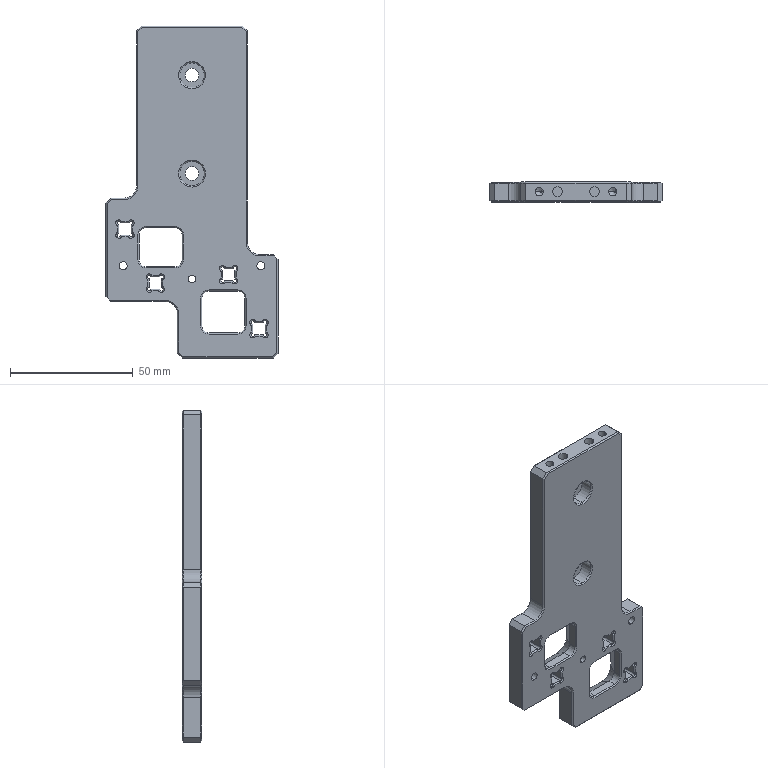Part | SolidWorks | features MoveFace 9, Chamfer 5, Cut 4, HoleWzd 4, Fillet 2, DelFace 1, Extrusion 1, ICE 1 | 1 solid | 276 faces | box 70 x 8 x 135 mm | volume 46021 mm3 | plane 129 | cone 90 | cylinder 57 | commonest cylinder face diameters 1.5 x24 3.3 x8 6 x8 10 x7 4 x4 5.5 x4